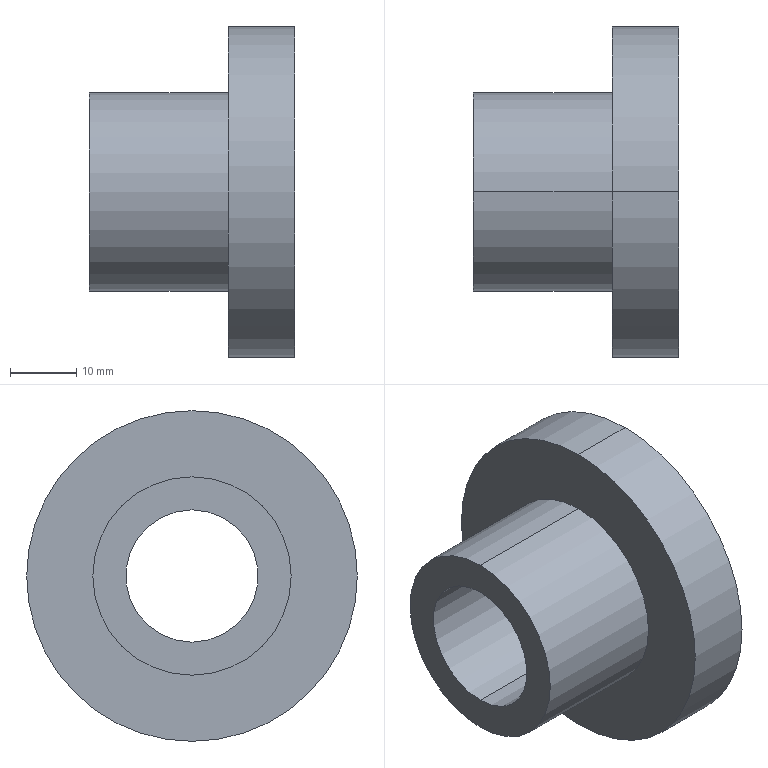Part | SolidWorks | features Chamfer 1, Revolution 1 | 1 solid | 11 faces | box 31 x 50 x 50 mm | volume 24606 mm3 | cylinder 6 | plane 3 | cone 2 | commonest cylinder face diameters 20 x2 30 x2 50 x2
STEP:
#1=CARTESIAN_POINT('',(8.218,0.,10.));
#2=VERTEX_POINT('',#1);
#3=CARTESIAN_POINT('',(8.218,0.,-10.));
#4=VERTEX_POINT('',#3);
#5=CARTESIAN_POINT('',(8.218,0.,0.));
#6=DIRECTION('',(1.,0.,0.));
#7=DIRECTION('',(0.,0.,1.));
#8=AXIS2_PLACEMENT_3D('',#5,#6,#7);
#9=CIRCLE('',#8,10.);
#10=EDGE_CURVE('',#2,#4,#9,.T.);
#11=ORIENTED_EDGE('',*,*,#10,.F.);
#12=CARTESIAN_POINT('',(10.218,0.,12.));
#13=VERTEX_POINT('',#12);
#14=CARTESIAN_POINT('',(10.218,0.,12.));
#15=DIRECTION('',(0.7071,0.,0.7071));
#16=VECTOR('',#15,1000.);
#17=LINE('',#14,#16);
#18=EDGE_CURVE('',#2,#13,#17,.T.);
#19=ORIENTED_EDGE('',*,*,#18,.T.);
#20=CARTESIAN_POINT('',(10.218,0.,-12.));
#21=VERTEX_POINT('',#20);
#22=CARTESIAN_POINT('',(10.218,0.,0.));
#23=DIRECTION('',(-1.,0.,0.));
#24=DIRECTION('',(0.,0.,1.));
#25=AXIS2_PLACEMENT_3D('',#22,#23,#24);
#26=CIRCLE('',#25,12.);
#27=EDGE_CURVE('',#21,#13,#26,.T.);
#28=ORIENTED_EDGE('',*,*,#27,.F.);
#29=CARTESIAN_POINT('',(10.218,0.,-12.));
#30=DIRECTION('',(0.7071,0.,-0.7071));
#31=VECTOR('',#30,1000.);
#32=LINE('',#29,#31);
#33=EDGE_CURVE('',#4,#21,#32,.T.);
#34=ORIENTED_EDGE('',*,*,#33,.F.);
#35=EDGE_LOOP('',(#11,#19,#28,#34));
#36=FACE_OUTER_BOUND('',#35,.T.);
#37=CARTESIAN_POINT('',(10.218,0.,0.));
#38=DIRECTION('',(1.,0.,0.));
#39=DIRECTION('',(0.,0.,-1.));
#40=AXIS2_PLACEMENT_3D('',#37,#38,#39);
#41=CONICAL_SURFACE('',#40,12.,0.7854);
#42=ADVANCED_FACE('',(#36),#41,.F.);
#43=CARTESIAN_POINT('',(0.2176,0.,15.));
#44=VERTEX_POINT('',#43);
#45=CARTESIAN_POINT('',(0.2176,0.,-15.));
#46=VERTEX_POINT('',#45);
#47=CARTESIAN_POINT('',(0.2176,0.,0.));
#48=DIRECTION('',(-1.,0.,0.));
#49=DIRECTION('',(0.,0.,1.));
#50=AXIS2_PLACEMENT_3D('',#47,#48,#49);
#51=CIRCLE('',#50,15.);
#52=EDGE_CURVE('',#44,#46,#51,.T.);
#53=ORIENTED_EDGE('',*,*,#52,.T.);
#54=CARTESIAN_POINT('',(-20.782,0.,-15.));
#55=VERTEX_POINT('',#54);
#56=CARTESIAN_POINT('',(-31.663,0.,-15.));
#57=DIRECTION('',(-1.,0.,0.));
#58=VECTOR('',#57,1000.);
#59=LINE('',#56,#58);
#60=EDGE_CURVE('',#46,#55,#59,.T.);
#61=ORIENTED_EDGE('',*,*,#60,.T.);
#62=CARTESIAN_POINT('',(-20.782,0.,15.));
#63=VERTEX_POINT('',#62);
#64=CARTESIAN_POINT('',(-20.782,0.,0.));
#65=DIRECTION('',(-1.,0.,0.));
#66=DIRECTION('',(0.,0.,1.));
#67=AXIS2_PLACEMENT_3D('',#64,#65,#66);
#68=CIRCLE('',#67,15.);
#69=EDGE_CURVE('',#63,#55,#68,.T.);
#70=ORIENTED_EDGE('',*,*,#69,.F.);
#71=CARTESIAN_POINT('',(-31.663,0.,15.));
#72=DIRECTION('',(-1.,0.,0.));
#73=VECTOR('',#72,1000.);
#74=LINE('',#71,#73);
#75=EDGE_CURVE('',#44,#63,#74,.T.);
#76=ORIENTED_EDGE('',*,*,#75,.F.);
#77=EDGE_LOOP('',(#53,#61,#70,#76));
#78=FACE_OUTER_BOUND('',#77,.T.);
#79=CARTESIAN_POINT('',(-31.663,0.,0.));
#80=DIRECTION('',(-1.,0.,0.));
#81=DIRECTION('',(0.,0.,1.));
#82=AXIS2_PLACEMENT_3D('',#79,#80,#81);
#83=CYLINDRICAL_SURFACE('',#82,15.);
#84=ADVANCED_FACE('',(#78),#83,.T.);
#85=CARTESIAN_POINT('',(10.218,0.,25.));
#86=VERTEX_POINT('',#85);
#87=CARTESIAN_POINT('',(10.218,0.,-25.));
#88=VERTEX_POINT('',#87);
#89=CARTESIAN_POINT('',(10.218,0.,0.));
#90=DIRECTION('',(-1.,0.,0.));
#91=DIRECTION('',(0.,0.,1.));
#92=AXIS2_PLACEMENT_3D('',#89,#90,#91);
#93=CIRCLE('',#92,25.);
#94=EDGE_CURVE('',#86,#88,#93,.T.);
#95=ORIENTED_EDGE('',*,*,#94,.T.);
#96=CARTESIAN_POINT('',(0.2176,0.,-25.));
#97=VERTEX_POINT('',#96);
#98=CARTESIAN_POINT('',(-31.663,0.,-25.));
#99=DIRECTION('',(-1.,0.,0.));
#100=VECTOR('',#99,1000.);
#101=LINE('',#98,#100);
#102=EDGE_CURVE('',#88,#97,#101,.T.);
#103=ORIENTED_EDGE('',*,*,#102,.T.);
#104=CARTESIAN_POINT('',(0.2176,0.,25.));
#105=VERTEX_POINT('',#104);
#106=CARTESIAN_POINT('',(0.2176,0.,0.));
#107=DIRECTION('',(-1.,0.,0.));
#108=DIRECTION('',(0.,0.,1.));
#109=AXIS2_PLACEMENT_3D('',#106,#107,#108);
#110=CIRCLE('',#109,25.);
#111=EDGE_CURVE('',#105,#97,#110,.T.);
#112=ORIENTED_EDGE('',*,*,#111,.F.);
#113=CARTESIAN_POINT('',(-31.663,0.,25.));
#114=DIRECTION('',(-1.,0.,0.));
#115=VECTOR('',#114,1000.);
#116=LINE('',#113,#115);
#117=EDGE_CURVE('',#86,#105,#116,.T.);
#118=ORIENTED_EDGE('',*,*,#117,.F.);
#119=EDGE_LOOP('',(#95,#103,#112,#118));
#120=FACE_OUTER_BOUND('',#119,.T.);
#121=CARTESIAN_POINT('',(-31.663,0.,0.));
#122=DIRECTION('',(-1.,0.,0.));
#123=DIRECTION('',(0.,0.,1.));
#124=AXIS2_PLACEMENT_3D('',#121,#122,#123);
#125=CYLINDRICAL_SURFACE('',#124,25.);
#126=ADVANCED_FACE('',(#120),#125,.T.);
#127=ORIENTED_EDGE('',*,*,#10,.T.);
#128=CARTESIAN_POINT('',(-20.782,0.,-10.));
#129=VERTEX_POINT('',#128);
#130=CARTESIAN_POINT('',(-31.663,0.,-10.));
#131=DIRECTION('',(-1.,0.,0.));
#132=VECTOR('',#131,1000.);
#133=LINE('',#130,#132);
#134=EDGE_CURVE('',#4,#129,#133,.T.);
#135=ORIENTED_EDGE('',*,*,#134,.T.);
#136=CARTESIAN_POINT('',(-20.782,0.,10.));
#137=VERTEX_POINT('',#136);
#138=CARTESIAN_POINT('',(-20.782,0.,0.));
#139=DIRECTION('',(-1.,0.,0.));
#140=DIRECTION('',(0.,0.,1.));
#141=AXIS2_PLACEMENT_3D('',#138,#139,#140);
#142=CIRCLE('',#141,10.);
#143=EDGE_CURVE('',#129,#137,#142,.T.);
#144=ORIENTED_EDGE('',*,*,#143,.T.);
#145=CARTESIAN_POINT('',(-31.663,0.,10.));
#146=DIRECTION('',(-1.,0.,0.));
#147=VECTOR('',#146,1000.);
#148=LINE('',#145,#147);
#149=EDGE_CURVE('',#2,#137,#148,.T.);
#150=ORIENTED_EDGE('',*,*,#149,.F.);
#151=EDGE_LOOP('',(#127,#135,#144,#150));
#152=FACE_OUTER_BOUND('',#151,.T.);
#153=CARTESIAN_POINT('',(-31.663,0.,0.));
#154=DIRECTION('',(-1.,0.,0.));
#155=DIRECTION('',(0.,0.,1.));
#156=AXIS2_PLACEMENT_3D('',#153,#154,#155);
#157=CYLINDRICAL_SURFACE('',#156,10.);
#158=ADVANCED_FACE('',(#152),#157,.F.);
#159=CARTESIAN_POINT('',(-20.782,0.,0.));
#160=DIRECTION('',(-1.,0.,0.));
#161=DIRECTION('',(0.,0.,1.));
#162=AXIS2_PLACEMENT_3D('',#159,#160,#161);
#163=CIRCLE('',#162,10.);
#164=EDGE_CURVE('',#137,#129,#163,.T.);
#165=ORIENTED_EDGE('',*,*,#164,.F.);
#166=ORIENTED_EDGE('',*,*,#143,.F.);
#167=EDGE_LOOP('',(#165,#166));
#168=FACE_BOUND('',#167,.T.);
#169=ORIENTED_EDGE('',*,*,#69,.T.);
#170=CARTESIAN_POINT('',(-20.782,0.,0.));
#171=DIRECTION('',(-1.,0.,0.));
#172=DIRECTION('',(0.,0.,1.));
#173=AXIS2_PLACEMENT_3D('',#170,#171,#172);
#174=CIRCLE('',#173,15.);
#175=EDGE_CURVE('',#55,#63,#174,.T.);
#176=ORIENTED_EDGE('',*,*,#175,.T.);
#177=EDGE_LOOP('',(#169,#176));
#178=FACE_OUTER_BOUND('',#177,.T.);
#179=CARTESIAN_POINT('',(-20.782,15.,0.));
#180=DIRECTION('',(1.,0.,0.));
#181=DIRECTION('',(0.,0.,-1.));
#182=AXIS2_PLACEMENT_3D('',#179,#180,#181);
#183=PLANE('',#182);
#184=ADVANCED_FACE('',(#168,#178),#183,.F.);
#185=ORIENTED_EDGE('',*,*,#134,.F.);
#186=CARTESIAN_POINT('',(8.218,0.,0.));
#187=DIRECTION('',(1.,0.,0.));
#188=DIRECTION('',(0.,0.,1.));
#189=AXIS2_PLACEMENT_3D('',#186,#187,#188);
#190=CIRCLE('',#189,10.);
#191=EDGE_CURVE('',#4,#2,#190,.T.);
#192=ORIENTED_EDGE('',*,*,#191,.T.);
#193=ORIENTED_EDGE('',*,*,#149,.T.);
#194=ORIENTED_EDGE('',*,*,#164,.T.);
#195=EDGE_LOOP('',(#185,#192,#193,#194));
#196=FACE_OUTER_BOUND('',#195,.T.);
#197=CARTESIAN_POINT('',(-31.663,0.,0.));
#198=DIRECTION('',(-1.,0.,0.));
#199=DIRECTION('',(0.,0.,1.));
#200=AXIS2_PLACEMENT_3D('',#197,#198,#199);
#201=CYLINDRICAL_SURFACE('',#200,10.);
#202=ADVANCED_FACE('',(#196),#201,.F.);
#203=ORIENTED_EDGE('',*,*,#27,.T.);
#204=CARTESIAN_POINT('',(10.218,0.,0.));
#205=DIRECTION('',(-1.,0.,0.));
#206=DIRECTION('',(0.,0.,1.));
#207=AXIS2_PLACEMENT_3D('',#204,#205,#206);
#208=CIRCLE('',#207,12.);
#209=EDGE_CURVE('',#13,#21,#208,.T.);
#210=ORIENTED_EDGE('',*,*,#209,.T.);
#211=EDGE_LOOP('',(#203,#210));
#212=FACE_BOUND('',#211,.T.);
#213=ORIENTED_EDGE('',*,*,#94,.F.);
#214=CARTESIAN_POINT('',(10.218,0.,0.));
#215=DIRECTION('',(-1.,0.,0.));
#216=DIRECTION('',(0.,0.,1.));
#217=AXIS2_PLACEMENT_3D('',#214,#215,#216);
#218=CIRCLE('',#217,25.);
#219=EDGE_CURVE('',#88,#86,#218,.T.);
#220=ORIENTED_EDGE('',*,*,#219,.F.);
#221=EDGE_LOOP('',(#213,#220));
#222=FACE_OUTER_BOUND('',#221,.T.);
#223=CARTESIAN_POINT('',(10.218,10.,0.));
#224=DIRECTION('',(-1.,0.,0.));
#225=DIRECTION('',(0.,0.,1.));
#226=AXIS2_PLACEMENT_3D('',#223,#224,#225);
#227=PLANE('',#226);
#228=ADVANCED_FACE('',(#212,#222),#227,.F.);
#229=ORIENTED_EDGE('',*,*,#102,.F.);
#230=ORIENTED_EDGE('',*,*,#219,.T.);
#231=ORIENTED_EDGE('',*,*,#117,.T.);
#232=CARTESIAN_POINT('',(0.2176,0.,0.));
#233=DIRECTION('',(-1.,0.,0.));
#234=DIRECTION('',(0.,0.,1.));
#235=AXIS2_PLACEMENT_3D('',#232,#233,#234);
#236=CIRCLE('',#235,25.);
#237=EDGE_CURVE('',#97,#105,#236,.T.);
#238=ORIENTED_EDGE('',*,*,#237,.F.);
#239=EDGE_LOOP('',(#229,#230,#231,#238));
#240=FACE_OUTER_BOUND('',#239,.T.);
#241=CARTESIAN_POINT('',(-31.663,0.,0.));
#242=DIRECTION('',(-1.,0.,0.));
#243=DIRECTION('',(0.,0.,1.));
#244=AXIS2_PLACEMENT_3D('',#241,#242,#243);
#245=CYLINDRICAL_SURFACE('',#244,25.);
#246=ADVANCED_FACE('',(#240),#245,.T.);
#247=ORIENTED_EDGE('',*,*,#52,.F.);
#248=CARTESIAN_POINT('',(0.2176,0.,0.));
#249=DIRECTION('',(-1.,0.,0.));
#250=DIRECTION('',(0.,0.,1.));
#251=AXIS2_PLACEMENT_3D('',#248,#249,#250);
#252=CIRCLE('',#251,15.);
#253=EDGE_CURVE('',#46,#44,#252,.T.);
#254=ORIENTED_EDGE('',*,*,#253,.F.);
#255=EDGE_LOOP('',(#247,#254));
#256=FACE_BOUND('',#255,.T.);
#257=ORIENTED_EDGE('',*,*,#111,.T.);
#258=ORIENTED_EDGE('',*,*,#237,.T.);
#259=EDGE_LOOP('',(#257,#258));
#260=FACE_OUTER_BOUND('',#259,.T.);
#261=CARTESIAN_POINT('',(0.2176,25.,0.));
#262=DIRECTION('',(1.,0.,0.));
#263=DIRECTION('',(0.,0.,-1.));
#264=AXIS2_PLACEMENT_3D('',#261,#262,#263);
#265=PLANE('',#264);
#266=ADVANCED_FACE('',(#256,#260),#265,.F.);
#267=ORIENTED_EDGE('',*,*,#60,.F.);
#268=ORIENTED_EDGE('',*,*,#253,.T.);
#269=ORIENTED_EDGE('',*,*,#75,.T.);
#270=ORIENTED_EDGE('',*,*,#175,.F.);
#271=EDGE_LOOP('',(#267,#268,#269,#270));
#272=FACE_OUTER_BOUND('',#271,.T.);
#273=CARTESIAN_POINT('',(-31.663,0.,0.));
#274=DIRECTION('',(-1.,0.,0.));
#275=DIRECTION('',(0.,0.,1.));
#276=AXIS2_PLACEMENT_3D('',#273,#274,#275);
#277=CYLINDRICAL_SURFACE('',#276,15.);
#278=ADVANCED_FACE('',(#272),#277,.T.);
#279=ORIENTED_EDGE('',*,*,#18,.F.);
#280=ORIENTED_EDGE('',*,*,#191,.F.);
#281=ORIENTED_EDGE('',*,*,#33,.T.);
#282=ORIENTED_EDGE('',*,*,#209,.F.);
#283=EDGE_LOOP('',(#279,#280,#281,#282));
#284=FACE_OUTER_BOUND('',#283,.T.);
#285=CARTESIAN_POINT('',(10.218,0.,0.));
#286=DIRECTION('',(1.,0.,0.));
#287=DIRECTION('',(0.,0.,-1.));
#288=AXIS2_PLACEMENT_3D('',#285,#286,#287);
#289=CONICAL_SURFACE('',#288,12.,0.7854);
#290=ADVANCED_FACE('',(#284),#289,.F.);
#291=CLOSED_SHELL('',(#42,#84,#126,#158,#184,#202,#228,#246,#266,#278,#290));
#292=MANIFOLD_SOLID_BREP('',#291);
#293=CARTESIAN_POINT('',(0.,0.,0.));
#294=DIRECTION('',(0.,0.,1.));
#295=DIRECTION('',(1.,0.,0.));
#296=AXIS2_PLACEMENT_3D('',#293,#294,#295);
#297=(LENGTH_UNIT()NAMED_UNIT(*)SI_UNIT(.MILLI.,.METRE.));
#298=UNCERTAINTY_MEASURE_WITH_UNIT(LENGTH_MEASURE(0.00001),#297,'','');
#299=(NAMED_UNIT(*)PLANE_ANGLE_UNIT()SI_UNIT($,.RADIAN.));
#300=(NAMED_UNIT(*)SI_UNIT($,.STERADIAN.)SOLID_ANGLE_UNIT());
#301=(GEOMETRIC_REPRESENTATION_CONTEXT(3)GLOBAL_UNCERTAINTY_ASSIGNED_CONTEXT((#298))GLOBAL_UNIT_ASSIGNED_CONTEXT((#297,#299,#300))REPRESENTATION_CONTEXT('',''));
#302=ADVANCED_BREP_SHAPE_REPRESENTATION('',(#292,#296),#301);